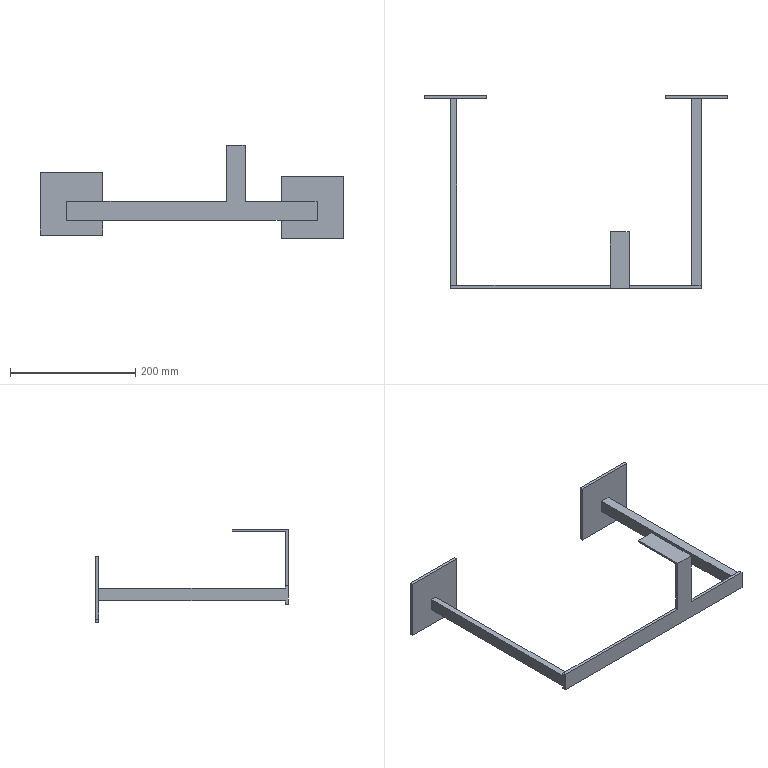Part | SolidWorks | features ICE 5, BaseBody 1, MoveFace 1 | 1 solid | 34 faces | box 485.708 x 308 x 149.774 mm | volume 313754 mm3 | plane 34
STEP:
#1=CARTESIAN_POINT('',(116.168,-5.,15.));
#2=VERTEX_POINT('',#1);
#3=CARTESIAN_POINT('',(116.168,0.,15.));
#4=VERTEX_POINT('',#3);
#5=CARTESIAN_POINT('',(116.168,0.,15.));
#6=DIRECTION('',(0.,1.,0.));
#7=VECTOR('',#6,1000.);
#8=LINE('',#5,#7);
#9=EDGE_CURVE('',#2,#4,#8,.T.);
#10=ORIENTED_EDGE('',*,*,#9,.F.);
#11=CARTESIAN_POINT('',(231.168,-5.,15.));
#12=VERTEX_POINT('',#11);
#13=CARTESIAN_POINT('',(0.,-5.,15.));
#14=DIRECTION('',(-1.,0.,0.));
#15=VECTOR('',#14,1000.);
#16=LINE('',#13,#15);
#17=EDGE_CURVE('',#12,#2,#16,.T.);
#18=ORIENTED_EDGE('',*,*,#17,.F.);
#19=CARTESIAN_POINT('',(231.168,0.,15.));
#20=VERTEX_POINT('',#19);
#21=CARTESIAN_POINT('',(231.168,-5.,15.));
#22=DIRECTION('',(0.,-1.,0.));
#23=VECTOR('',#22,1000.);
#24=LINE('',#21,#23);
#25=EDGE_CURVE('',#20,#12,#24,.T.);
#26=ORIENTED_EDGE('',*,*,#25,.F.);
#27=CARTESIAN_POINT('',(-168.832,0.,15.));
#28=DIRECTION('',(1.,0.,0.));
#29=VECTOR('',#28,1000.);
#30=LINE('',#27,#29);
#31=EDGE_CURVE('',#4,#20,#30,.T.);
#32=ORIENTED_EDGE('',*,*,#31,.F.);
#33=EDGE_LOOP('',(#10,#18,#26,#32));
#34=FACE_OUTER_BOUND('',#33,.T.);
#35=CARTESIAN_POINT('',(-168.832,-5.,15.));
#36=DIRECTION('',(0.,0.,-1.));
#37=DIRECTION('',(-1.,0.,0.));
#38=AXIS2_PLACEMENT_3D('',#35,#36,#37);
#39=PLANE('',#38);
#40=ADVANCED_FACE('',(#34),#39,.F.);
#41=CARTESIAN_POINT('',(86.168,85.,105.));
#42=VERTEX_POINT('',#41);
#43=CARTESIAN_POINT('',(86.168,-5.,105.));
#44=VERTEX_POINT('',#43);
#45=CARTESIAN_POINT('',(86.168,-5.,105.));
#46=DIRECTION('',(0.,-1.,0.));
#47=VECTOR('',#46,1000.);
#48=LINE('',#45,#47);
#49=EDGE_CURVE('',#42,#44,#48,.T.);
#50=ORIENTED_EDGE('',*,*,#49,.T.);
#51=CARTESIAN_POINT('',(116.168,-5.,105.));
#52=VERTEX_POINT('',#51);
#53=CARTESIAN_POINT('',(116.168,-5.,105.));
#54=DIRECTION('',(1.,0.,0.));
#55=VECTOR('',#54,1000.);
#56=LINE('',#53,#55);
#57=EDGE_CURVE('',#44,#52,#56,.T.);
#58=ORIENTED_EDGE('',*,*,#57,.T.);
#59=CARTESIAN_POINT('',(116.168,85.,105.));
#60=VERTEX_POINT('',#59);
#61=CARTESIAN_POINT('',(116.168,-5.,105.));
#62=DIRECTION('',(0.,1.,0.));
#63=VECTOR('',#62,1000.);
#64=LINE('',#61,#63);
#65=EDGE_CURVE('',#52,#60,#64,.T.);
#66=ORIENTED_EDGE('',*,*,#65,.T.);
#67=CARTESIAN_POINT('',(116.168,85.,105.));
#68=DIRECTION('',(-1.,0.,0.));
#69=VECTOR('',#68,1000.);
#70=LINE('',#67,#69);
#71=EDGE_CURVE('',#60,#42,#70,.T.);
#72=ORIENTED_EDGE('',*,*,#71,.T.);
#73=EDGE_LOOP('',(#50,#58,#66,#72));
#74=FACE_OUTER_BOUND('',#73,.T.);
#75=CARTESIAN_POINT('',(-168.832,-5.,105.));
#76=DIRECTION('',(0.,0.,-1.));
#77=DIRECTION('',(-1.,0.,0.));
#78=AXIS2_PLACEMENT_3D('',#75,#76,#77);
#79=PLANE('',#78);
#80=ADVANCED_FACE('',(#74),#79,.F.);
#81=CARTESIAN_POINT('',(86.168,0.,15.));
#82=VERTEX_POINT('',#81);
#83=CARTESIAN_POINT('',(86.168,-5.,15.));
#84=VERTEX_POINT('',#83);
#85=CARTESIAN_POINT('',(86.168,0.,15.));
#86=DIRECTION('',(0.,-1.,0.));
#87=VECTOR('',#86,1000.);
#88=LINE('',#85,#87);
#89=EDGE_CURVE('',#82,#84,#88,.T.);
#90=ORIENTED_EDGE('',*,*,#89,.F.);
#91=CARTESIAN_POINT('',(-168.832,0.,15.));
#92=VERTEX_POINT('',#91);
#93=CARTESIAN_POINT('',(-168.832,0.,15.));
#94=DIRECTION('',(1.,0.,0.));
#95=VECTOR('',#94,1000.);
#96=LINE('',#93,#95);
#97=EDGE_CURVE('',#92,#82,#96,.T.);
#98=ORIENTED_EDGE('',*,*,#97,.F.);
#99=CARTESIAN_POINT('',(-168.832,-5.,15.));
#100=VERTEX_POINT('',#99);
#101=CARTESIAN_POINT('',(-168.832,-5.,15.));
#102=DIRECTION('',(0.,1.,0.));
#103=VECTOR('',#102,1000.);
#104=LINE('',#101,#103);
#105=EDGE_CURVE('',#100,#92,#104,.T.);
#106=ORIENTED_EDGE('',*,*,#105,.F.);
#107=CARTESIAN_POINT('',(0.,-5.,15.));
#108=DIRECTION('',(-1.,0.,0.));
#109=VECTOR('',#108,1000.);
#110=LINE('',#107,#109);
#111=EDGE_CURVE('',#84,#100,#110,.T.);
#112=ORIENTED_EDGE('',*,*,#111,.F.);
#113=EDGE_LOOP('',(#90,#98,#106,#112));
#114=FACE_OUTER_BOUND('',#113,.T.);
#115=CARTESIAN_POINT('',(-168.832,-5.,15.));
#116=DIRECTION('',(0.,0.,-1.));
#117=DIRECTION('',(-1.,0.,0.));
#118=AXIS2_PLACEMENT_3D('',#115,#116,#117);
#119=PLANE('',#118);
#120=ADVANCED_FACE('',(#114),#119,.F.);
#121=ORIENTED_EDGE('',*,*,#17,.T.);
#122=CARTESIAN_POINT('',(116.168,-5.,105.));
#123=DIRECTION('',(0.,0.,-1.));
#124=VECTOR('',#123,1000.);
#125=LINE('',#122,#124);
#126=EDGE_CURVE('',#52,#2,#125,.T.);
#127=ORIENTED_EDGE('',*,*,#126,.F.);
#128=ORIENTED_EDGE('',*,*,#57,.F.);
#129=CARTESIAN_POINT('',(86.168,-5.,105.));
#130=DIRECTION('',(0.,0.,-1.));
#131=VECTOR('',#130,1000.);
#132=LINE('',#129,#131);
#133=EDGE_CURVE('',#44,#84,#132,.T.);
#134=ORIENTED_EDGE('',*,*,#133,.T.);
#135=ORIENTED_EDGE('',*,*,#111,.T.);
#136=CARTESIAN_POINT('',(-168.832,-5.,-15.));
#137=VERTEX_POINT('',#136);
#138=CARTESIAN_POINT('',(-168.832,-5.,0.));
#139=DIRECTION('',(0.,0.,-1.));
#140=VECTOR('',#139,1000.);
#141=LINE('',#138,#140);
#142=EDGE_CURVE('',#100,#137,#141,.T.);
#143=ORIENTED_EDGE('',*,*,#142,.T.);
#144=CARTESIAN_POINT('',(231.168,-5.,-15.));
#145=VERTEX_POINT('',#144);
#146=CARTESIAN_POINT('',(0.,-5.,-15.));
#147=DIRECTION('',(1.,0.,0.));
#148=VECTOR('',#147,1000.);
#149=LINE('',#146,#148);
#150=EDGE_CURVE('',#137,#145,#149,.T.);
#151=ORIENTED_EDGE('',*,*,#150,.T.);
#152=CARTESIAN_POINT('',(231.168,-5.,0.));
#153=DIRECTION('',(0.,0.,1.));
#154=VECTOR('',#153,1000.);
#155=LINE('',#152,#154);
#156=EDGE_CURVE('',#145,#12,#155,.T.);
#157=ORIENTED_EDGE('',*,*,#156,.T.);
#158=EDGE_LOOP('',(#121,#127,#128,#134,#135,#143,#151,#157));
#159=FACE_OUTER_BOUND('',#158,.T.);
#160=CARTESIAN_POINT('',(0.,-5.,0.));
#161=DIRECTION('',(0.,-1.,0.));
#162=DIRECTION('',(0.,0.,-1.));
#163=AXIS2_PLACEMENT_3D('',#160,#161,#162);
#164=PLANE('',#163);
#165=ADVANCED_FACE('',(#159),#164,.T.);
#166=CARTESIAN_POINT('',(231.168,0.,10.299));
#167=VERTEX_POINT('',#166);
#168=CARTESIAN_POINT('',(231.168,0.,15.));
#169=DIRECTION('',(0.,0.,-1.));
#170=VECTOR('',#169,1000.);
#171=LINE('',#168,#170);
#172=EDGE_CURVE('',#20,#167,#171,.T.);
#173=ORIENTED_EDGE('',*,*,#172,.F.);
#174=ORIENTED_EDGE('',*,*,#25,.T.);
#175=ORIENTED_EDGE('',*,*,#156,.F.);
#176=CARTESIAN_POINT('',(231.168,0.,-15.));
#177=VERTEX_POINT('',#176);
#178=CARTESIAN_POINT('',(231.168,-5.,-15.));
#179=DIRECTION('',(0.,-1.,0.));
#180=VECTOR('',#179,1000.);
#181=LINE('',#178,#180);
#182=EDGE_CURVE('',#177,#145,#181,.T.);
#183=ORIENTED_EDGE('',*,*,#182,.F.);
#184=CARTESIAN_POINT('',(231.168,0.,-9.701));
#185=VERTEX_POINT('',#184);
#186=CARTESIAN_POINT('',(231.168,0.,15.));
#187=DIRECTION('',(0.,0.,-1.));
#188=VECTOR('',#187,1000.);
#189=LINE('',#186,#188);
#190=EDGE_CURVE('',#185,#177,#189,.T.);
#191=ORIENTED_EDGE('',*,*,#190,.F.);
#192=CARTESIAN_POINT('',(231.168,298.,-9.701));
#193=VERTEX_POINT('',#192);
#194=CARTESIAN_POINT('',(231.168,-5.,-9.701));
#195=DIRECTION('',(0.,-1.,0.));
#196=VECTOR('',#195,1000.);
#197=LINE('',#194,#196);
#198=EDGE_CURVE('',#193,#185,#197,.T.);
#199=ORIENTED_EDGE('',*,*,#198,.F.);
#200=CARTESIAN_POINT('',(231.168,298.,10.299));
#201=VERTEX_POINT('',#200);
#202=CARTESIAN_POINT('',(231.168,298.,15.));
#203=DIRECTION('',(0.,0.,-1.));
#204=VECTOR('',#203,1000.);
#205=LINE('',#202,#204);
#206=EDGE_CURVE('',#201,#193,#205,.T.);
#207=ORIENTED_EDGE('',*,*,#206,.F.);
#208=CARTESIAN_POINT('',(231.168,-5.,10.299));
#209=DIRECTION('',(0.,1.,0.));
#210=VECTOR('',#209,1000.);
#211=LINE('',#208,#210);
#212=EDGE_CURVE('',#167,#201,#211,.T.);
#213=ORIENTED_EDGE('',*,*,#212,.F.);
#214=EDGE_LOOP('',(#173,#174,#175,#183,#191,#199,#207,#213));
#215=FACE_OUTER_BOUND('',#214,.T.);
#216=CARTESIAN_POINT('',(231.168,-5.,15.));
#217=DIRECTION('',(-1.,0.,0.));
#218=DIRECTION('',(0.,0.,1.));
#219=AXIS2_PLACEMENT_3D('',#216,#217,#218);
#220=PLANE('',#219);
#221=ADVANCED_FACE('',(#215),#220,.F.);
#222=CARTESIAN_POINT('',(-168.832,0.,-15.));
#223=VERTEX_POINT('',#222);
#224=CARTESIAN_POINT('',(-168.832,0.,-15.));
#225=DIRECTION('',(-1.,0.,0.));
#226=VECTOR('',#225,1000.);
#227=LINE('',#224,#226);
#228=EDGE_CURVE('',#177,#223,#227,.T.);
#229=ORIENTED_EDGE('',*,*,#228,.F.);
#230=ORIENTED_EDGE('',*,*,#182,.T.);
#231=ORIENTED_EDGE('',*,*,#150,.F.);
#232=CARTESIAN_POINT('',(-168.832,-5.,-15.));
#233=DIRECTION('',(0.,-1.,0.));
#234=VECTOR('',#233,1000.);
#235=LINE('',#232,#234);
#236=EDGE_CURVE('',#223,#137,#235,.T.);
#237=ORIENTED_EDGE('',*,*,#236,.F.);
#238=EDGE_LOOP('',(#229,#230,#231,#237));
#239=FACE_OUTER_BOUND('',#238,.T.);
#240=CARTESIAN_POINT('',(-168.832,-5.,-15.));
#241=DIRECTION('',(0.,0.,1.));
#242=DIRECTION('',(1.,0.,0.));
#243=AXIS2_PLACEMENT_3D('',#240,#241,#242);
#244=PLANE('',#243);
#245=ADVANCED_FACE('',(#239),#244,.F.);
#246=CARTESIAN_POINT('',(-168.832,298.,10.299));
#247=VERTEX_POINT('',#246);
#248=CARTESIAN_POINT('',(-168.832,0.,10.299));
#249=VERTEX_POINT('',#248);
#250=CARTESIAN_POINT('',(-168.832,-5.,10.299));
#251=DIRECTION('',(0.,-1.,0.));
#252=VECTOR('',#251,1000.);
#253=LINE('',#250,#252);
#254=EDGE_CURVE('',#247,#249,#253,.T.);
#255=ORIENTED_EDGE('',*,*,#254,.F.);
#256=CARTESIAN_POINT('',(-168.832,298.,-9.701));
#257=VERTEX_POINT('',#256);
#258=CARTESIAN_POINT('',(-168.832,298.,15.));
#259=DIRECTION('',(0.,0.,1.));
#260=VECTOR('',#259,1000.);
#261=LINE('',#258,#260);
#262=EDGE_CURVE('',#257,#247,#261,.T.);
#263=ORIENTED_EDGE('',*,*,#262,.F.);
#264=CARTESIAN_POINT('',(-168.832,0.,-9.701));
#265=VERTEX_POINT('',#264);
#266=CARTESIAN_POINT('',(-168.832,-5.,-9.701));
#267=DIRECTION('',(0.,1.,0.));
#268=VECTOR('',#267,1000.);
#269=LINE('',#266,#268);
#270=EDGE_CURVE('',#265,#257,#269,.T.);
#271=ORIENTED_EDGE('',*,*,#270,.F.);
#272=CARTESIAN_POINT('',(-168.832,0.,15.));
#273=DIRECTION('',(0.,0.,1.));
#274=VECTOR('',#273,1000.);
#275=LINE('',#272,#274);
#276=EDGE_CURVE('',#223,#265,#275,.T.);
#277=ORIENTED_EDGE('',*,*,#276,.F.);
#278=ORIENTED_EDGE('',*,*,#236,.T.);
#279=ORIENTED_EDGE('',*,*,#142,.F.);
#280=ORIENTED_EDGE('',*,*,#105,.T.);
#281=CARTESIAN_POINT('',(-168.832,0.,15.));
#282=DIRECTION('',(0.,0.,1.));
#283=VECTOR('',#282,1000.);
#284=LINE('',#281,#283);
#285=EDGE_CURVE('',#249,#92,#284,.T.);
#286=ORIENTED_EDGE('',*,*,#285,.F.);
#287=EDGE_LOOP('',(#255,#263,#271,#277,#278,#279,#280,#286));
#288=FACE_OUTER_BOUND('',#287,.T.);
#289=CARTESIAN_POINT('',(-168.832,-5.,15.));
#290=DIRECTION('',(1.,0.,0.));
#291=DIRECTION('',(0.,0.,-1.));
#292=AXIS2_PLACEMENT_3D('',#289,#290,#291);
#293=PLANE('',#292);
#294=ADVANCED_FACE('',(#288),#293,.F.);
#295=CARTESIAN_POINT('',(216.168,0.,10.299));
#296=VERTEX_POINT('',#295);
#297=CARTESIAN_POINT('',(0.,0.,10.299));
#298=DIRECTION('',(1.,0.,0.));
#299=VECTOR('',#298,1000.);
#300=LINE('',#297,#299);
#301=EDGE_CURVE('',#296,#167,#300,.T.);
#302=ORIENTED_EDGE('',*,*,#301,.F.);
#303=CARTESIAN_POINT('',(-159.065,0.,10.299));
#304=VERTEX_POINT('',#303);
#305=CARTESIAN_POINT('',(0.,0.,10.299));
#306=DIRECTION('',(1.,0.,0.));
#307=VECTOR('',#306,1000.);
#308=LINE('',#305,#307);
#309=EDGE_CURVE('',#304,#296,#308,.T.);
#310=ORIENTED_EDGE('',*,*,#309,.F.);
#311=CARTESIAN_POINT('',(0.,0.,10.299));
#312=DIRECTION('',(1.,0.,0.));
#313=VECTOR('',#312,1000.);
#314=LINE('',#311,#313);
#315=EDGE_CURVE('',#249,#304,#314,.T.);
#316=ORIENTED_EDGE('',*,*,#315,.F.);
#317=ORIENTED_EDGE('',*,*,#285,.T.);
#318=ORIENTED_EDGE('',*,*,#97,.T.);
#319=CARTESIAN_POINT('',(86.168,0.,102.));
#320=VERTEX_POINT('',#319);
#321=CARTESIAN_POINT('',(86.168,0.,105.));
#322=DIRECTION('',(0.,0.,-1.));
#323=VECTOR('',#322,1000.);
#324=LINE('',#321,#323);
#325=EDGE_CURVE('',#320,#82,#324,.T.);
#326=ORIENTED_EDGE('',*,*,#325,.F.);
#327=CARTESIAN_POINT('',(116.168,0.,102.));
#328=VERTEX_POINT('',#327);
#329=CARTESIAN_POINT('',(0.,0.,102.));
#330=DIRECTION('',(-1.,0.,0.));
#331=VECTOR('',#330,1000.);
#332=LINE('',#329,#331);
#333=EDGE_CURVE('',#328,#320,#332,.T.);
#334=ORIENTED_EDGE('',*,*,#333,.F.);
#335=CARTESIAN_POINT('',(116.168,0.,102.));
#336=CARTESIAN_POINT('',(116.168,0.,73.));
#337=CARTESIAN_POINT('',(116.168,0.,44.));
#338=CARTESIAN_POINT('',(116.168,0.,15.));
#339=B_SPLINE_CURVE_WITH_KNOTS('',3,(#335,#336,#337,#338),.UNSPECIFIED.,.F.,.F.,(4,4),(0.,1.),.UNSPECIFIED.);
#340=EDGE_CURVE('',#328,#4,#339,.T.);
#341=ORIENTED_EDGE('',*,*,#340,.T.);
#342=ORIENTED_EDGE('',*,*,#31,.T.);
#343=ORIENTED_EDGE('',*,*,#172,.T.);
#344=EDGE_LOOP('',(#302,#310,#316,#317,#318,#326,#334,#341,#342,#343));
#345=FACE_OUTER_BOUND('',#344,.T.);
#346=CARTESIAN_POINT('',(0.,0.,0.));
#347=DIRECTION('',(0.,-1.,0.));
#348=DIRECTION('',(0.,0.,-1.));
#349=AXIS2_PLACEMENT_3D('',#346,#347,#348);
#350=PLANE('',#349);
#351=ADVANCED_FACE('',(#345),#350,.F.);
#352=ORIENTED_EDGE('',*,*,#301,.T.);
#353=ORIENTED_EDGE('',*,*,#212,.T.);
#354=CARTESIAN_POINT('',(216.168,298.,10.299));
#355=VERTEX_POINT('',#354);
#356=CARTESIAN_POINT('',(216.168,298.,10.299));
#357=DIRECTION('',(1.,0.,0.));
#358=VECTOR('',#357,1000.);
#359=LINE('',#356,#358);
#360=EDGE_CURVE('',#355,#201,#359,.T.);
#361=ORIENTED_EDGE('',*,*,#360,.F.);
#362=CARTESIAN_POINT('',(216.168,298.,10.299));
#363=DIRECTION('',(0.,1.,0.));
#364=VECTOR('',#363,1000.);
#365=LINE('',#362,#364);
#366=EDGE_CURVE('',#296,#355,#365,.T.);
#367=ORIENTED_EDGE('',*,*,#366,.F.);
#368=EDGE_LOOP('',(#352,#353,#361,#367));
#369=FACE_OUTER_BOUND('',#368,.T.);
#370=CARTESIAN_POINT('',(216.168,298.,10.299));
#371=DIRECTION('',(0.,0.,-1.));
#372=DIRECTION('',(-1.,0.,0.));
#373=AXIS2_PLACEMENT_3D('',#370,#371,#372);
#374=PLANE('',#373);
#375=ADVANCED_FACE('',(#369),#374,.F.);
#376=ORIENTED_EDGE('',*,*,#190,.T.);
#377=ORIENTED_EDGE('',*,*,#228,.T.);
#378=ORIENTED_EDGE('',*,*,#276,.T.);
#379=CARTESIAN_POINT('',(-159.065,0.,-9.701));
#380=VERTEX_POINT('',#379);
#381=CARTESIAN_POINT('',(0.,0.,-9.701));
#382=DIRECTION('',(-1.,0.,0.));
#383=VECTOR('',#382,1000.);
#384=LINE('',#381,#383);
#385=EDGE_CURVE('',#380,#265,#384,.T.);
#386=ORIENTED_EDGE('',*,*,#385,.F.);
#387=CARTESIAN_POINT('',(216.168,0.,-9.701));
#388=VERTEX_POINT('',#387);
#389=CARTESIAN_POINT('',(0.,0.,-9.701));
#390=DIRECTION('',(-1.,0.,0.));
#391=VECTOR('',#390,1000.);
#392=LINE('',#389,#391);
#393=EDGE_CURVE('',#388,#380,#392,.T.);
#394=ORIENTED_EDGE('',*,*,#393,.F.);
#395=CARTESIAN_POINT('',(0.,0.,-9.701));
#396=DIRECTION('',(-1.,0.,0.));
#397=VECTOR('',#396,1000.);
#398=LINE('',#395,#397);
#399=EDGE_CURVE('',#185,#388,#398,.T.);
#400=ORIENTED_EDGE('',*,*,#399,.F.);
#401=EDGE_LOOP('',(#376,#377,#378,#386,#394,#400));
#402=FACE_OUTER_BOUND('',#401,.T.);
#403=CARTESIAN_POINT('',(0.,0.,0.));
#404=DIRECTION('',(0.,-1.,0.));
#405=DIRECTION('',(0.,0.,-1.));
#406=AXIS2_PLACEMENT_3D('',#403,#404,#405);
#407=PLANE('',#406);
#408=ADVANCED_FACE('',(#402),#407,.F.);
#409=ORIENTED_EDGE('',*,*,#399,.T.);
#410=CARTESIAN_POINT('',(216.168,298.,-9.701));
#411=VERTEX_POINT('',#410);
#412=CARTESIAN_POINT('',(216.168,298.,-9.701));
#413=DIRECTION('',(0.,-1.,0.));
#414=VECTOR('',#413,1000.);
#415=LINE('',#412,#414);
#416=EDGE_CURVE('',#411,#388,#415,.T.);
#417=ORIENTED_EDGE('',*,*,#416,.F.);
#418=CARTESIAN_POINT('',(216.168,298.,-9.701));
#419=DIRECTION('',(-1.,0.,0.));
#420=VECTOR('',#419,1000.);
#421=LINE('',#418,#420);
#422=EDGE_CURVE('',#193,#411,#421,.T.);
#423=ORIENTED_EDGE('',*,*,#422,.F.);
#424=ORIENTED_EDGE('',*,*,#198,.T.);
#425=EDGE_LOOP('',(#409,#417,#423,#424));
#426=FACE_OUTER_BOUND('',#425,.T.);
#427=CARTESIAN_POINT('',(216.168,298.,-9.701));
#428=DIRECTION('',(0.,0.,1.));
#429=DIRECTION('',(1.,0.,0.));
#430=AXIS2_PLACEMENT_3D('',#427,#428,#429);
#431=PLANE('',#430);
#432=ADVANCED_FACE('',(#426),#431,.F.);
#433=CARTESIAN_POINT('',(216.168,298.,0.));
#434=DIRECTION('',(0.,0.,-1.));
#435=VECTOR('',#434,1000.);
#436=LINE('',#433,#435);
#437=EDGE_CURVE('',#355,#411,#436,.T.);
#438=ORIENTED_EDGE('',*,*,#437,.F.);
#439=ORIENTED_EDGE('',*,*,#360,.T.);
#440=ORIENTED_EDGE('',*,*,#206,.T.);
#441=ORIENTED_EDGE('',*,*,#422,.T.);
#442=EDGE_LOOP('',(#438,#439,#440,#441));
#443=FACE_BOUND('',#442,.T.);
#444=CARTESIAN_POINT('',(274.106,298.,-44.774));
#445=VERTEX_POINT('',#444);
#446=CARTESIAN_POINT('',(174.106,298.,-44.774));
#447=VERTEX_POINT('',#446);
#448=CARTESIAN_POINT('',(0.,298.,-44.774));
#449=DIRECTION('',(-1.,0.,0.));
#450=VECTOR('',#449,1000.);
#451=LINE('',#448,#450);
#452=EDGE_CURVE('',#445,#447,#451,.T.);
#453=ORIENTED_EDGE('',*,*,#452,.F.);
#454=CARTESIAN_POINT('',(274.106,298.,55.226));
#455=VERTEX_POINT('',#454);
#456=CARTESIAN_POINT('',(274.106,298.,0.));
#457=DIRECTION('',(0.,0.,-1.));
#458=VECTOR('',#457,1000.);
#459=LINE('',#456,#458);
#460=EDGE_CURVE('',#455,#445,#459,.T.);
#461=ORIENTED_EDGE('',*,*,#460,.F.);
#462=CARTESIAN_POINT('',(174.106,298.,55.226));
#463=VERTEX_POINT('',#462);
#464=CARTESIAN_POINT('',(0.,298.,55.226));
#465=DIRECTION('',(1.,0.,0.));
#466=VECTOR('',#465,1000.);
#467=LINE('',#464,#466);
#468=EDGE_CURVE('',#463,#455,#467,.T.);
#469=ORIENTED_EDGE('',*,*,#468,.F.);
#470=CARTESIAN_POINT('',(174.106,298.,0.));
#471=DIRECTION('',(0.,0.,1.));
#472=VECTOR('',#471,1000.);
#473=LINE('',#470,#472);
#474=EDGE_CURVE('',#447,#463,#473,.T.);
#475=ORIENTED_EDGE('',*,*,#474,.F.);
#476=EDGE_LOOP('',(#453,#461,#469,#475));
#477=FACE_OUTER_BOUND('',#476,.T.);
#478=CARTESIAN_POINT('',(0.,298.,0.));
#479=DIRECTION('',(0.,1.,0.));
#480=DIRECTION('',(0.,0.,1.));
#481=AXIS2_PLACEMENT_3D('',#478,#479,#480);
#482=PLANE('',#481);
#483=ADVANCED_FACE('',(#443,#477),#482,.F.);
#484=ORIENTED_EDGE('',*,*,#315,.T.);
#485=CARTESIAN_POINT('',(-159.065,298.,10.299));
#486=VERTEX_POINT('',#485);
#487=CARTESIAN_POINT('',(-159.065,298.,10.299));
#488=DIRECTION('',(0.,-1.,0.));
#489=VECTOR('',#488,1000.);
#490=LINE('',#487,#489);
#491=EDGE_CURVE('',#486,#304,#490,.T.);
#492=ORIENTED_EDGE('',*,*,#491,.F.);
#493=CARTESIAN_POINT('',(-168.832,298.,10.299));
#494=DIRECTION('',(1.,0.,0.));
#495=VECTOR('',#494,1000.);
#496=LINE('',#493,#495);
#497=EDGE_CURVE('',#247,#486,#496,.T.);
#498=ORIENTED_EDGE('',*,*,#497,.F.);
#499=ORIENTED_EDGE('',*,*,#254,.T.);
#500=EDGE_LOOP('',(#484,#492,#498,#499));
#501=FACE_OUTER_BOUND('',#500,.T.);
#502=CARTESIAN_POINT('',(-168.832,298.,10.299));
#503=DIRECTION('',(0.,0.,-1.));
#504=DIRECTION('',(-1.,0.,0.));
#505=AXIS2_PLACEMENT_3D('',#502,#503,#504);
#506=PLANE('',#505);
#507=ADVANCED_FACE('',(#501),#506,.F.);
#508=ORIENTED_EDGE('',*,*,#262,.T.);
#509=ORIENTED_EDGE('',*,*,#497,.T.);
#510=CARTESIAN_POINT('',(-159.065,298.,-9.701));
#511=VERTEX_POINT('',#510);
#512=CARTESIAN_POINT('',(-159.065,298.,0.));
#513=DIRECTION('',(0.,0.,1.));
#514=VECTOR('',#513,1000.);
#515=LINE('',#512,#514);
#516=EDGE_CURVE('',#511,#486,#515,.T.);
#517=ORIENTED_EDGE('',*,*,#516,.F.);
#518=CARTESIAN_POINT('',(0.,298.,-9.701));
#519=DIRECTION('',(1.,0.,0.));
#520=VECTOR('',#519,1000.);
#521=LINE('',#518,#520);
#522=EDGE_CURVE('',#257,#511,#521,.T.);
#523=ORIENTED_EDGE('',*,*,#522,.F.);
#524=EDGE_LOOP('',(#508,#509,#517,#523));
#525=FACE_BOUND('',#524,.T.);
#526=CARTESIAN_POINT('',(-111.603,298.,-38.716));
#527=VERTEX_POINT('',#526);
#528=CARTESIAN_POINT('',(-211.603,298.,-38.716));
#529=VERTEX_POINT('',#528);
#530=CARTESIAN_POINT('',(0.,298.,-38.716));
#531=DIRECTION('',(-1.,0.,0.));
#532=VECTOR('',#531,1000.);
#533=LINE('',#530,#532);
#534=EDGE_CURVE('',#527,#529,#533,.T.);
#535=ORIENTED_EDGE('',*,*,#534,.F.);
#536=CARTESIAN_POINT('',(-111.603,298.,61.284));
#537=VERTEX_POINT('',#536);
#538=CARTESIAN_POINT('',(-111.603,298.,0.));
#539=DIRECTION('',(0.,0.,-1.));
#540=VECTOR('',#539,1000.);
#541=LINE('',#538,#540);
#542=EDGE_CURVE('',#537,#527,#541,.T.);
#543=ORIENTED_EDGE('',*,*,#542,.F.);
#544=CARTESIAN_POINT('',(-211.603,298.,61.284));
#545=VERTEX_POINT('',#544);
#546=CARTESIAN_POINT('',(0.,298.,61.284));
#547=DIRECTION('',(1.,0.,0.));
#548=VECTOR('',#547,1000.);
#549=LINE('',#546,#548);
#550=EDGE_CURVE('',#545,#537,#549,.T.);
#551=ORIENTED_EDGE('',*,*,#550,.F.);
#552=CARTESIAN_POINT('',(-211.603,298.,0.));
#553=DIRECTION('',(0.,0.,1.));
#554=VECTOR('',#553,1000.);
#555=LINE('',#552,#554);
#556=EDGE_CURVE('',#529,#545,#555,.T.);
#557=ORIENTED_EDGE('',*,*,#556,.F.);
#558=EDGE_LOOP('',(#535,#543,#551,#557));
#559=FACE_OUTER_BOUND('',#558,.T.);
#560=CARTESIAN_POINT('',(0.,298.,0.));
#561=DIRECTION('',(0.,1.,0.));
#562=DIRECTION('',(0.,0.,1.));
#563=AXIS2_PLACEMENT_3D('',#560,#561,#562);
#564=PLANE('',#563);
#565=ADVANCED_FACE('',(#525,#559),#564,.F.);
#566=ORIENTED_EDGE('',*,*,#385,.T.);
#567=ORIENTED_EDGE('',*,*,#270,.T.);
#568=ORIENTED_EDGE('',*,*,#522,.T.);
#569=CARTESIAN_POINT('',(-159.065,298.,-9.701));
#570=DIRECTION('',(0.,1.,0.));
#571=VECTOR('',#570,1000.);
#572=LINE('',#569,#571);
#573=EDGE_CURVE('',#380,#511,#572,.T.);
#574=ORIENTED_EDGE('',*,*,#573,.F.);
#575=EDGE_LOOP('',(#566,#567,#568,#574));
#576=FACE_OUTER_BOUND('',#575,.T.);
#577=CARTESIAN_POINT('',(-168.832,298.,-9.701));
#578=DIRECTION('',(0.,0.,1.));
#579=DIRECTION('',(1.,0.,0.));
#580=AXIS2_PLACEMENT_3D('',#577,#578,#579);
#581=PLANE('',#580);
#582=ADVANCED_FACE('',(#576),#581,.F.);
#583=CARTESIAN_POINT('',(-159.065,-2.,10.299));
#584=VERTEX_POINT('',#583);
#585=CARTESIAN_POINT('',(216.168,-2.,10.299));
#586=VERTEX_POINT('',#585);
#587=CARTESIAN_POINT('',(231.168,-2.,10.299));
#588=DIRECTION('',(1.,0.,0.));
#589=VECTOR('',#588,1000.);
#590=LINE('',#587,#589);
#591=EDGE_CURVE('',#584,#586,#590,.T.);
#592=ORIENTED_EDGE('',*,*,#591,.F.);
#593=CARTESIAN_POINT('',(-159.065,0.,10.299));
#594=DIRECTION('',(0.,-1.,0.));
#595=VECTOR('',#594,1000.);
#596=LINE('',#593,#595);
#597=EDGE_CURVE('',#304,#584,#596,.T.);
#598=ORIENTED_EDGE('',*,*,#597,.F.);
#599=ORIENTED_EDGE('',*,*,#309,.T.);
#600=CARTESIAN_POINT('',(216.168,0.,10.299));
#601=DIRECTION('',(0.,1.,0.));
#602=VECTOR('',#601,1000.);
#603=LINE('',#600,#602);
#604=EDGE_CURVE('',#586,#296,#603,.T.);
#605=ORIENTED_EDGE('',*,*,#604,.F.);
#606=EDGE_LOOP('',(#592,#598,#599,#605));
#607=FACE_OUTER_BOUND('',#606,.T.);
#608=CARTESIAN_POINT('',(231.168,0.,10.299));
#609=DIRECTION('',(0.,0.,1.));
#610=DIRECTION('',(1.,0.,0.));
#611=AXIS2_PLACEMENT_3D('',#608,#609,#610);
#612=PLANE('',#611);
#613=ADVANCED_FACE('',(#607),#612,.F.);
#614=ORIENTED_EDGE('',*,*,#604,.T.);
#615=ORIENTED_EDGE('',*,*,#366,.T.);
#616=ORIENTED_EDGE('',*,*,#437,.T.);
#617=ORIENTED_EDGE('',*,*,#416,.T.);
#618=CARTESIAN_POINT('',(216.168,-2.,-9.701));
#619=VERTEX_POINT('',#618);
#620=CARTESIAN_POINT('',(216.168,298.,-9.701));
#621=DIRECTION('',(0.,1.,0.));
#622=VECTOR('',#621,1000.);
#623=LINE('',#620,#622);
#624=EDGE_CURVE('',#619,#388,#623,.T.);
#625=ORIENTED_EDGE('',*,*,#624,.F.);
#626=CARTESIAN_POINT('',(216.168,-2.,-9.701));
#627=DIRECTION('',(0.,0.,-1.));
#628=VECTOR('',#627,1000.);
#629=LINE('',#626,#628);
#630=EDGE_CURVE('',#586,#619,#629,.T.);
#631=ORIENTED_EDGE('',*,*,#630,.F.);
#632=EDGE_LOOP('',(#614,#615,#616,#617,#625,#631));
#633=FACE_OUTER_BOUND('',#632,.T.);
#634=CARTESIAN_POINT('',(216.168,298.,-9.701));
#635=DIRECTION('',(1.,0.,0.));
#636=DIRECTION('',(0.,0.,-1.));
#637=AXIS2_PLACEMENT_3D('',#634,#635,#636);
#638=PLANE('',#637);
#639=ADVANCED_FACE('',(#633),#638,.F.);
#640=CARTESIAN_POINT('',(-159.065,-2.,-9.701));
#641=VERTEX_POINT('',#640);
#642=CARTESIAN_POINT('',(231.168,-2.,-9.701));
#643=DIRECTION('',(-1.,0.,0.));
#644=VECTOR('',#643,1000.);
#645=LINE('',#642,#644);
#646=EDGE_CURVE('',#619,#641,#645,.T.);
#647=ORIENTED_EDGE('',*,*,#646,.F.);
#648=ORIENTED_EDGE('',*,*,#624,.T.);
#649=ORIENTED_EDGE('',*,*,#393,.T.);
#650=CARTESIAN_POINT('',(-159.065,0.,-9.701));
#651=DIRECTION('',(0.,1.,0.));
#652=VECTOR('',#651,1000.);
#653=LINE('',#650,#652);
#654=EDGE_CURVE('',#641,#380,#653,.T.);
#655=ORIENTED_EDGE('',*,*,#654,.F.);
#656=EDGE_LOOP('',(#647,#648,#649,#655));
#657=FACE_OUTER_BOUND('',#656,.T.);
#658=CARTESIAN_POINT('',(231.168,0.,-9.701));
#659=DIRECTION('',(0.,0.,-1.));
#660=DIRECTION('',(-1.,0.,0.));
#661=AXIS2_PLACEMENT_3D('',#658,#659,#660);
#662=PLANE('',#661);
#663=ADVANCED_FACE('',(#657),#662,.F.);
#664=CARTESIAN_POINT('',(174.106,303.,55.226));
#665=VERTEX_POINT('',#664);
#666=CARTESIAN_POINT('',(174.106,303.,55.226));
#667=DIRECTION('',(0.,-1.,0.));
#668=VECTOR('',#667,1000.);
#669=LINE('',#666,#668);
#670=EDGE_CURVE('',#665,#463,#669,.T.);
#671=ORIENTED_EDGE('',*,*,#670,.F.);
#672=CARTESIAN_POINT('',(174.106,303.,-44.774));
#673=VERTEX_POINT('',#672);
#674=CARTESIAN_POINT('',(174.106,303.,-44.774));
#675=DIRECTION('',(0.,0.,1.));
#676=VECTOR('',#675,1000.);
#677=LINE('',#674,#676);
#678=EDGE_CURVE('',#673,#665,#677,.T.);
#679=ORIENTED_EDGE('',*,*,#678,.F.);
#680=CARTESIAN_POINT('',(174.106,303.,-44.774));
#681=DIRECTION('',(0.,1.,0.));
#682=VECTOR('',#681,1000.);
#683=LINE('',#680,#682);
#684=EDGE_CURVE('',#447,#673,#683,.T.);
#685=ORIENTED_EDGE('',*,*,#684,.F.);
#686=ORIENTED_EDGE('',*,*,#474,.T.);
#687=EDGE_LOOP('',(#671,#679,#685,#686));
#688=FACE_OUTER_BOUND('',#687,.T.);
#689=CARTESIAN_POINT('',(174.106,303.,-44.774));
#690=DIRECTION('',(1.,0.,0.));
#691=DIRECTION('',(0.,0.,-1.));
#692=AXIS2_PLACEMENT_3D('',#689,#690,#691);
#693=PLANE('',#692);
#694=ADVANCED_FACE('',(#688),#693,.F.);
#695=ORIENTED_EDGE('',*,*,#684,.T.);
#696=CARTESIAN_POINT('',(274.106,303.,-44.774));
#697=VERTEX_POINT('',#696);
#698=CARTESIAN_POINT('',(174.106,303.,-44.774));
#699=DIRECTION('',(-1.,0.,0.));
#700=VECTOR('',#699,1000.);
#701=LINE('',#698,#700);
#702=EDGE_CURVE('',#697,#673,#701,.T.);
#703=ORIENTED_EDGE('',*,*,#702,.F.);
#704=CARTESIAN_POINT('',(274.106,303.,-44.774));
#705=DIRECTION('',(0.,1.,0.));
#706=VECTOR('',#705,1000.);
#707=LINE('',#704,#706);
#708=EDGE_CURVE('',#445,#697,#707,.T.);
#709=ORIENTED_EDGE('',*,*,#708,.F.);
#710=ORIENTED_EDGE('',*,*,#452,.T.);
#711=EDGE_LOOP('',(#695,#703,#709,#710));
#712=FACE_OUTER_BOUND('',#711,.T.);
#713=CARTESIAN_POINT('',(174.106,303.,-44.774));
#714=DIRECTION('',(0.,0.,1.));
#715=DIRECTION('',(1.,0.,0.));
#716=AXIS2_PLACEMENT_3D('',#713,#714,#715);
#717=PLANE('',#716);
#718=ADVANCED_FACE('',(#712),#717,.F.);
#719=ORIENTED_EDGE('',*,*,#708,.T.);
#720=CARTESIAN_POINT('',(274.106,303.,55.226));
#721=VERTEX_POINT('',#720);
#722=CARTESIAN_POINT('',(274.106,303.,-44.774));
#723=DIRECTION('',(0.,0.,-1.));
#724=VECTOR('',#723,1000.);
#725=LINE('',#722,#724);
#726=EDGE_CURVE('',#721,#697,#725,.T.);
#727=ORIENTED_EDGE('',*,*,#726,.F.);
#728=CARTESIAN_POINT('',(274.106,303.,55.226));
#729=DIRECTION('',(0.,1.,0.));
#730=VECTOR('',#729,1000.);
#731=LINE('',#728,#730);
#732=EDGE_CURVE('',#455,#721,#731,.T.);
#733=ORIENTED_EDGE('',*,*,#732,.F.);
#734=ORIENTED_EDGE('',*,*,#460,.T.);
#735=EDGE_LOOP('',(#719,#727,#733,#734));
#736=FACE_OUTER_BOUND('',#735,.T.);
#737=CARTESIAN_POINT('',(274.106,303.,-44.774));
#738=DIRECTION('',(-1.,0.,0.));
#739=DIRECTION('',(0.,0.,1.));
#740=AXIS2_PLACEMENT_3D('',#737,#738,#739);
#741=PLANE('',#740);
#742=ADVANCED_FACE('',(#736),#741,.F.);
#743=ORIENTED_EDGE('',*,*,#732,.T.);
#744=CARTESIAN_POINT('',(174.106,303.,55.226));
#745=DIRECTION('',(1.,0.,0.));
#746=VECTOR('',#745,1000.);
#747=LINE('',#744,#746);
#748=EDGE_CURVE('',#665,#721,#747,.T.);
#749=ORIENTED_EDGE('',*,*,#748,.F.);
#750=ORIENTED_EDGE('',*,*,#670,.T.);
#751=ORIENTED_EDGE('',*,*,#468,.T.);
#752=EDGE_LOOP('',(#743,#749,#750,#751));
#753=FACE_OUTER_BOUND('',#752,.T.);
#754=CARTESIAN_POINT('',(174.106,303.,55.226));
#755=DIRECTION('',(0.,0.,-1.));
#756=DIRECTION('',(-1.,0.,0.));
#757=AXIS2_PLACEMENT_3D('',#754,#755,#756);
#758=PLANE('',#757);
#759=ADVANCED_FACE('',(#753),#758,.F.);
#760=ORIENTED_EDGE('',*,*,#654,.T.);
#761=ORIENTED_EDGE('',*,*,#573,.T.);
#762=ORIENTED_EDGE('',*,*,#516,.T.);
#763=ORIENTED_EDGE('',*,*,#491,.T.);
#764=ORIENTED_EDGE('',*,*,#597,.T.);
#765=CARTESIAN_POINT('',(-159.065,-2.,-9.701));
#766=DIRECTION('',(0.,0.,1.));
#767=VECTOR('',#766,1000.);
#768=LINE('',#765,#767);
#769=EDGE_CURVE('',#641,#584,#768,.T.);
#770=ORIENTED_EDGE('',*,*,#769,.F.);
#771=EDGE_LOOP('',(#760,#761,#762,#763,#764,#770));
#772=FACE_OUTER_BOUND('',#771,.T.);
#773=CARTESIAN_POINT('',(-159.065,298.,-9.701));
#774=DIRECTION('',(-1.,0.,0.));
#775=DIRECTION('',(0.,0.,1.));
#776=AXIS2_PLACEMENT_3D('',#773,#774,#775);
#777=PLANE('',#776);
#778=ADVANCED_FACE('',(#772),#777,.F.);
#779=CARTESIAN_POINT('',(-211.603,303.,61.284));
#780=VERTEX_POINT('',#779);
#781=CARTESIAN_POINT('',(-211.603,303.,61.284));
#782=DIRECTION('',(0.,-1.,0.));
#783=VECTOR('',#782,1000.);
#784=LINE('',#781,#783);
#785=EDGE_CURVE('',#780,#545,#784,.T.);
#786=ORIENTED_EDGE('',*,*,#785,.F.);
#787=CARTESIAN_POINT('',(-211.603,303.,-38.716));
#788=VERTEX_POINT('',#787);
#789=CARTESIAN_POINT('',(-211.603,303.,-38.716));
#790=DIRECTION('',(0.,0.,1.));
#791=VECTOR('',#790,1000.);
#792=LINE('',#789,#791);
#793=EDGE_CURVE('',#788,#780,#792,.T.);
#794=ORIENTED_EDGE('',*,*,#793,.F.);
#795=CARTESIAN_POINT('',(-211.603,303.,-38.716));
#796=DIRECTION('',(0.,1.,0.));
#797=VECTOR('',#796,1000.);
#798=LINE('',#795,#797);
#799=EDGE_CURVE('',#529,#788,#798,.T.);
#800=ORIENTED_EDGE('',*,*,#799,.F.);
#801=ORIENTED_EDGE('',*,*,#556,.T.);
#802=EDGE_LOOP('',(#786,#794,#800,#801));
#803=FACE_OUTER_BOUND('',#802,.T.);
#804=CARTESIAN_POINT('',(-211.603,303.,-38.716));
#805=DIRECTION('',(1.,0.,0.));
#806=DIRECTION('',(0.,0.,-1.));
#807=AXIS2_PLACEMENT_3D('',#804,#805,#806);
#808=PLANE('',#807);
#809=ADVANCED_FACE('',(#803),#808,.F.);
#810=ORIENTED_EDGE('',*,*,#799,.T.);
#811=CARTESIAN_POINT('',(-111.603,303.,-38.716));
#812=VERTEX_POINT('',#811);
#813=CARTESIAN_POINT('',(-211.603,303.,-38.716));
#814=DIRECTION('',(-1.,0.,0.));
#815=VECTOR('',#814,1000.);
#816=LINE('',#813,#815);
#817=EDGE_CURVE('',#812,#788,#816,.T.);
#818=ORIENTED_EDGE('',*,*,#817,.F.);
#819=CARTESIAN_POINT('',(-111.603,303.,-38.716));
#820=DIRECTION('',(0.,1.,0.));
#821=VECTOR('',#820,1000.);
#822=LINE('',#819,#821);
#823=EDGE_CURVE('',#527,#812,#822,.T.);
#824=ORIENTED_EDGE('',*,*,#823,.F.);
#825=ORIENTED_EDGE('',*,*,#534,.T.);
#826=EDGE_LOOP('',(#810,#818,#824,#825));
#827=FACE_OUTER_BOUND('',#826,.T.);
#828=CARTESIAN_POINT('',(-211.603,303.,-38.716));
#829=DIRECTION('',(0.,0.,1.));
#830=DIRECTION('',(1.,0.,0.));
#831=AXIS2_PLACEMENT_3D('',#828,#829,#830);
#832=PLANE('',#831);
#833=ADVANCED_FACE('',(#827),#832,.F.);
#834=ORIENTED_EDGE('',*,*,#823,.T.);
#835=CARTESIAN_POINT('',(-111.603,303.,61.284));
#836=VERTEX_POINT('',#835);
#837=CARTESIAN_POINT('',(-111.603,303.,-38.716));
#838=DIRECTION('',(0.,0.,-1.));
#839=VECTOR('',#838,1000.);
#840=LINE('',#837,#839);
#841=EDGE_CURVE('',#836,#812,#840,.T.);
#842=ORIENTED_EDGE('',*,*,#841,.F.);
#843=CARTESIAN_POINT('',(-111.603,303.,61.284));
#844=DIRECTION('',(0.,1.,0.));
#845=VECTOR('',#844,1000.);
#846=LINE('',#843,#845);
#847=EDGE_CURVE('',#537,#836,#846,.T.);
#848=ORIENTED_EDGE('',*,*,#847,.F.);
#849=ORIENTED_EDGE('',*,*,#542,.T.);
#850=EDGE_LOOP('',(#834,#842,#848,#849));
#851=FACE_OUTER_BOUND('',#850,.T.);
#852=CARTESIAN_POINT('',(-111.603,303.,-38.716));
#853=DIRECTION('',(-1.,0.,0.));
#854=DIRECTION('',(0.,0.,1.));
#855=AXIS2_PLACEMENT_3D('',#852,#853,#854);
#856=PLANE('',#855);
#857=ADVANCED_FACE('',(#851),#856,.F.);
#858=ORIENTED_EDGE('',*,*,#847,.T.);
#859=CARTESIAN_POINT('',(-211.603,303.,61.284));
#860=DIRECTION('',(1.,0.,0.));
#861=VECTOR('',#860,1000.);
#862=LINE('',#859,#861);
#863=EDGE_CURVE('',#780,#836,#862,.T.);
#864=ORIENTED_EDGE('',*,*,#863,.F.);
#865=ORIENTED_EDGE('',*,*,#785,.T.);
#866=ORIENTED_EDGE('',*,*,#550,.T.);
#867=EDGE_LOOP('',(#858,#864,#865,#866));
#868=FACE_OUTER_BOUND('',#867,.T.);
#869=CARTESIAN_POINT('',(-211.603,303.,61.284));
#870=DIRECTION('',(0.,0.,-1.));
#871=DIRECTION('',(-1.,0.,0.));
#872=AXIS2_PLACEMENT_3D('',#869,#870,#871);
#873=PLANE('',#872);
#874=ADVANCED_FACE('',(#868),#873,.F.);
#875=ORIENTED_EDGE('',*,*,#630,.T.);
#876=ORIENTED_EDGE('',*,*,#646,.T.);
#877=ORIENTED_EDGE('',*,*,#769,.T.);
#878=ORIENTED_EDGE('',*,*,#591,.T.);
#879=EDGE_LOOP('',(#875,#876,#877,#878));
#880=FACE_OUTER_BOUND('',#879,.T.);
#881=CARTESIAN_POINT('',(231.168,-2.,-9.701));
#882=DIRECTION('',(0.,-1.,0.));
#883=DIRECTION('',(0.,0.,-1.));
#884=AXIS2_PLACEMENT_3D('',#881,#882,#883);
#885=PLANE('',#884);
#886=ADVANCED_FACE('',(#880),#885,.F.);
#887=ORIENTED_EDGE('',*,*,#726,.T.);
#888=ORIENTED_EDGE('',*,*,#702,.T.);
#889=ORIENTED_EDGE('',*,*,#678,.T.);
#890=ORIENTED_EDGE('',*,*,#748,.T.);
#891=EDGE_LOOP('',(#887,#888,#889,#890));
#892=FACE_OUTER_BOUND('',#891,.T.);
#893=CARTESIAN_POINT('',(0.,303.,0.));
#894=DIRECTION('',(0.,1.,0.));
#895=DIRECTION('',(0.,0.,1.));
#896=AXIS2_PLACEMENT_3D('',#893,#894,#895);
#897=PLANE('',#896);
#898=ADVANCED_FACE('',(#892),#897,.T.);
#899=ORIENTED_EDGE('',*,*,#841,.T.);
#900=ORIENTED_EDGE('',*,*,#817,.T.);
#901=ORIENTED_EDGE('',*,*,#793,.T.);
#902=ORIENTED_EDGE('',*,*,#863,.T.);
#903=EDGE_LOOP('',(#899,#900,#901,#902));
#904=FACE_OUTER_BOUND('',#903,.T.);
#905=CARTESIAN_POINT('',(0.,303.,0.));
#906=DIRECTION('',(0.,1.,0.));
#907=DIRECTION('',(0.,0.,1.));
#908=AXIS2_PLACEMENT_3D('',#905,#906,#907);
#909=PLANE('',#908);
#910=ADVANCED_FACE('',(#904),#909,.T.);
#911=ORIENTED_EDGE('',*,*,#65,.F.);
#912=ORIENTED_EDGE('',*,*,#126,.T.);
#913=ORIENTED_EDGE('',*,*,#9,.T.);
#914=ORIENTED_EDGE('',*,*,#340,.F.);
#915=CARTESIAN_POINT('',(116.168,85.,102.));
#916=VERTEX_POINT('',#915);
#917=CARTESIAN_POINT('',(116.168,-5.,102.));
#918=DIRECTION('',(0.,1.,0.));
#919=VECTOR('',#918,1000.);
#920=LINE('',#917,#919);
#921=EDGE_CURVE('',#328,#916,#920,.T.);
#922=ORIENTED_EDGE('',*,*,#921,.T.);
#923=CARTESIAN_POINT('',(116.168,85.,12.));
#924=DIRECTION('',(0.,0.,1.));
#925=VECTOR('',#924,1000.);
#926=LINE('',#923,#925);
#927=EDGE_CURVE('',#916,#60,#926,.T.);
#928=ORIENTED_EDGE('',*,*,#927,.T.);
#929=EDGE_LOOP('',(#911,#912,#913,#914,#922,#928));
#930=FACE_OUTER_BOUND('',#929,.T.);
#931=CARTESIAN_POINT('',(116.168,-5.,12.));
#932=DIRECTION('',(1.,0.,0.));
#933=DIRECTION('',(0.,0.,-1.));
#934=AXIS2_PLACEMENT_3D('',#931,#932,#933);
#935=PLANE('',#934);
#936=ADVANCED_FACE('',(#930),#935,.T.);
#937=CARTESIAN_POINT('',(86.168,85.,102.));
#938=VERTEX_POINT('',#937);
#939=CARTESIAN_POINT('',(86.168,-5.,102.));
#940=DIRECTION('',(0.,-1.,0.));
#941=VECTOR('',#940,1000.);
#942=LINE('',#939,#941);
#943=EDGE_CURVE('',#938,#320,#942,.T.);
#944=ORIENTED_EDGE('',*,*,#943,.T.);
#945=ORIENTED_EDGE('',*,*,#325,.T.);
#946=ORIENTED_EDGE('',*,*,#89,.T.);
#947=ORIENTED_EDGE('',*,*,#133,.F.);
#948=ORIENTED_EDGE('',*,*,#49,.F.);
#949=CARTESIAN_POINT('',(86.168,85.,12.));
#950=DIRECTION('',(0.,0.,1.));
#951=VECTOR('',#950,1000.);
#952=LINE('',#949,#951);
#953=EDGE_CURVE('',#938,#42,#952,.T.);
#954=ORIENTED_EDGE('',*,*,#953,.F.);
#955=EDGE_LOOP('',(#944,#945,#946,#947,#948,#954));
#956=FACE_OUTER_BOUND('',#955,.T.);
#957=CARTESIAN_POINT('',(86.168,-5.,12.));
#958=DIRECTION('',(-1.,0.,0.));
#959=DIRECTION('',(0.,0.,1.));
#960=AXIS2_PLACEMENT_3D('',#957,#958,#959);
#961=PLANE('',#960);
#962=ADVANCED_FACE('',(#956),#961,.T.);
#963=ORIENTED_EDGE('',*,*,#921,.F.);
#964=ORIENTED_EDGE('',*,*,#333,.T.);
#965=ORIENTED_EDGE('',*,*,#943,.F.);
#966=CARTESIAN_POINT('',(116.168,85.,102.));
#967=DIRECTION('',(-1.,0.,0.));
#968=VECTOR('',#967,1000.);
#969=LINE('',#966,#968);
#970=EDGE_CURVE('',#916,#938,#969,.T.);
#971=ORIENTED_EDGE('',*,*,#970,.F.);
#972=EDGE_LOOP('',(#963,#964,#965,#971));
#973=FACE_OUTER_BOUND('',#972,.T.);
#974=CARTESIAN_POINT('',(0.,0.,102.));
#975=DIRECTION('',(0.,0.,1.));
#976=DIRECTION('',(1.,0.,0.));
#977=AXIS2_PLACEMENT_3D('',#974,#975,#976);
#978=PLANE('',#977);
#979=ADVANCED_FACE('',(#973),#978,.F.);
#980=ORIENTED_EDGE('',*,*,#71,.F.);
#981=ORIENTED_EDGE('',*,*,#927,.F.);
#982=ORIENTED_EDGE('',*,*,#970,.T.);
#983=ORIENTED_EDGE('',*,*,#953,.T.);
#984=EDGE_LOOP('',(#980,#981,#982,#983));
#985=FACE_OUTER_BOUND('',#984,.T.);
#986=CARTESIAN_POINT('',(116.168,85.,12.));
#987=DIRECTION('',(0.,1.,0.));
#988=DIRECTION('',(0.,0.,1.));
#989=AXIS2_PLACEMENT_3D('',#986,#987,#988);
#990=PLANE('',#989);
#991=ADVANCED_FACE('',(#985),#990,.T.);
#992=CLOSED_SHELL('',(#40,#80,#120,#165,#221,#245,#294,#351,#375,#408,#432,#483,#507,#565,#582,#613,#639,#663,#694,#718,#742,#759,#778,#809,#833,#857,#874,#886,#898,#910,#936,#962,#979,#991));
#993=MANIFOLD_SOLID_BREP('',#992);
#994=CARTESIAN_POINT('',(0.,0.,0.));
#995=DIRECTION('',(0.,0.,1.));
#996=DIRECTION('',(1.,0.,0.));
#997=AXIS2_PLACEMENT_3D('',#994,#995,#996);
#998=(LENGTH_UNIT()NAMED_UNIT(*)SI_UNIT(.MILLI.,.METRE.));
#999=UNCERTAINTY_MEASURE_WITH_UNIT(LENGTH_MEASURE(0.00001),#998,'','');
#1000=(NAMED_UNIT(*)PLANE_ANGLE_UNIT()SI_UNIT($,.RADIAN.));
#1001=(NAMED_UNIT(*)SI_UNIT($,.STERADIAN.)SOLID_ANGLE_UNIT());
#1002=(GEOMETRIC_REPRESENTATION_CONTEXT(3)GLOBAL_UNCERTAINTY_ASSIGNED_CONTEXT((#999))GLOBAL_UNIT_ASSIGNED_CONTEXT((#998,#1000,#1001))REPRESENTATION_CONTEXT('',''));
#1003=ADVANCED_BREP_SHAPE_REPRESENTATION('',(#993,#997),#1002);